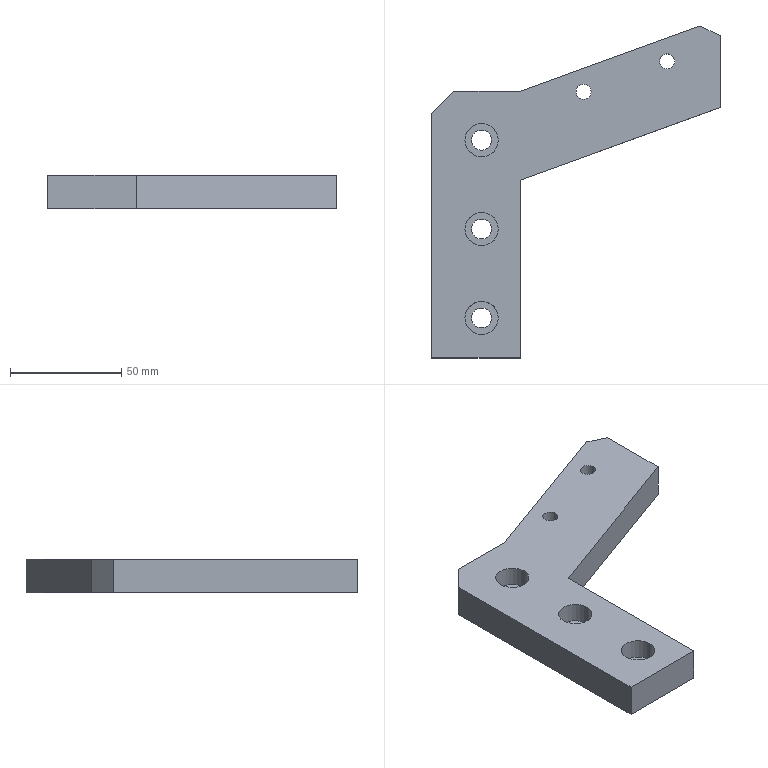Part | SolidWorks | features BaseBody 1 | 1 solid | 30 faces | box 130 x 149.337 x 15 mm | volume 117694 mm3 | cylinder 16 | plane 14 | commonest cylinder face diameters 9 x6 15 x6 6.8 x4
STEP:
#1=CARTESIAN_POINT('',(109.4,133.38,15.));
#2=VERTEX_POINT('',#1);
#3=CARTESIAN_POINT('',(102.6,133.38,15.));
#4=VERTEX_POINT('',#3);
#5=CARTESIAN_POINT('',(106.,133.38,15.));
#6=DIRECTION('',(0.,0.,-1.));
#7=DIRECTION('',(-1.,0.,0.));
#8=AXIS2_PLACEMENT_3D('',#5,#6,#7);
#9=CIRCLE('',#8,3.4);
#10=EDGE_CURVE('',#2,#4,#9,.T.);
#11=ORIENTED_EDGE('',*,*,#10,.F.);
#12=CARTESIAN_POINT('',(109.4,133.38,0.));
#13=VERTEX_POINT('',#12);
#14=CARTESIAN_POINT('',(109.4,133.38,0.));
#15=DIRECTION('',(0.,0.,-1.));
#16=VECTOR('',#15,1000.);
#17=LINE('',#14,#16);
#18=EDGE_CURVE('',#2,#13,#17,.T.);
#19=ORIENTED_EDGE('',*,*,#18,.T.);
#20=CARTESIAN_POINT('',(102.6,133.38,0.));
#21=VERTEX_POINT('',#20);
#22=CARTESIAN_POINT('',(106.,133.38,0.));
#23=DIRECTION('',(0.,0.,-1.));
#24=DIRECTION('',(-1.,0.,0.));
#25=AXIS2_PLACEMENT_3D('',#22,#23,#24);
#26=CIRCLE('',#25,3.4);
#27=EDGE_CURVE('',#13,#21,#26,.T.);
#28=ORIENTED_EDGE('',*,*,#27,.T.);
#29=CARTESIAN_POINT('',(102.6,133.38,0.));
#30=DIRECTION('',(0.,0.,-1.));
#31=VECTOR('',#30,1000.);
#32=LINE('',#29,#31);
#33=EDGE_CURVE('',#4,#21,#32,.T.);
#34=ORIENTED_EDGE('',*,*,#33,.F.);
#35=EDGE_LOOP('',(#11,#19,#28,#34));
#36=FACE_OUTER_BOUND('',#35,.T.);
#37=CARTESIAN_POINT('',(106.,133.38,0.));
#38=DIRECTION('',(0.,0.,-1.));
#39=DIRECTION('',(-1.,0.,0.));
#40=AXIS2_PLACEMENT_3D('',#37,#38,#39);
#41=CYLINDRICAL_SURFACE('',#40,3.4);
#42=ADVANCED_FACE('',(#36),#41,.F.);
#43=CARTESIAN_POINT('',(71.812,119.699,15.));
#44=VERTEX_POINT('',#43);
#45=CARTESIAN_POINT('',(65.012,119.699,15.));
#46=VERTEX_POINT('',#45);
#47=CARTESIAN_POINT('',(68.412,119.699,15.));
#48=DIRECTION('',(0.,0.,-1.));
#49=DIRECTION('',(-1.,0.,0.));
#50=AXIS2_PLACEMENT_3D('',#47,#48,#49);
#51=CIRCLE('',#50,3.4);
#52=EDGE_CURVE('',#44,#46,#51,.T.);
#53=ORIENTED_EDGE('',*,*,#52,.F.);
#54=CARTESIAN_POINT('',(71.812,119.699,0.));
#55=VERTEX_POINT('',#54);
#56=CARTESIAN_POINT('',(71.812,119.699,0.));
#57=DIRECTION('',(0.,0.,-1.));
#58=VECTOR('',#57,1000.);
#59=LINE('',#56,#58);
#60=EDGE_CURVE('',#44,#55,#59,.T.);
#61=ORIENTED_EDGE('',*,*,#60,.T.);
#62=CARTESIAN_POINT('',(65.012,119.699,0.));
#63=VERTEX_POINT('',#62);
#64=CARTESIAN_POINT('',(68.412,119.699,0.));
#65=DIRECTION('',(0.,0.,-1.));
#66=DIRECTION('',(-1.,0.,0.));
#67=AXIS2_PLACEMENT_3D('',#64,#65,#66);
#68=CIRCLE('',#67,3.4);
#69=EDGE_CURVE('',#55,#63,#68,.T.);
#70=ORIENTED_EDGE('',*,*,#69,.T.);
#71=CARTESIAN_POINT('',(65.012,119.699,0.));
#72=DIRECTION('',(0.,0.,-1.));
#73=VECTOR('',#72,1000.);
#74=LINE('',#71,#73);
#75=EDGE_CURVE('',#46,#63,#74,.T.);
#76=ORIENTED_EDGE('',*,*,#75,.F.);
#77=EDGE_LOOP('',(#53,#61,#70,#76));
#78=FACE_OUTER_BOUND('',#77,.T.);
#79=CARTESIAN_POINT('',(68.412,119.699,0.));
#80=DIRECTION('',(0.,0.,-1.));
#81=DIRECTION('',(-1.,0.,0.));
#82=AXIS2_PLACEMENT_3D('',#79,#80,#81);
#83=CYLINDRICAL_SURFACE('',#82,3.4);
#84=ADVANCED_FACE('',(#78),#83,.F.);
#85=CARTESIAN_POINT('',(15.,98.,6.));
#86=VERTEX_POINT('',#85);
#87=CARTESIAN_POINT('',(30.,98.,6.));
#88=VERTEX_POINT('',#87);
#89=CARTESIAN_POINT('',(22.5,98.,6.));
#90=DIRECTION('',(0.,0.,1.));
#91=DIRECTION('',(1.,0.,0.));
#92=AXIS2_PLACEMENT_3D('',#89,#90,#91);
#93=CIRCLE('',#92,7.5);
#94=EDGE_CURVE('',#86,#88,#93,.T.);
#95=ORIENTED_EDGE('',*,*,#94,.F.);
#96=CARTESIAN_POINT('',(15.,98.,15.));
#97=VERTEX_POINT('',#96);
#98=CARTESIAN_POINT('',(15.,98.,15.));
#99=DIRECTION('',(0.,0.,1.));
#100=VECTOR('',#99,1000.);
#101=LINE('',#98,#100);
#102=EDGE_CURVE('',#86,#97,#101,.T.);
#103=ORIENTED_EDGE('',*,*,#102,.T.);
#104=CARTESIAN_POINT('',(30.,98.,15.));
#105=VERTEX_POINT('',#104);
#106=CARTESIAN_POINT('',(22.5,98.,15.));
#107=DIRECTION('',(0.,0.,1.));
#108=DIRECTION('',(1.,0.,0.));
#109=AXIS2_PLACEMENT_3D('',#106,#107,#108);
#110=CIRCLE('',#109,7.5);
#111=EDGE_CURVE('',#97,#105,#110,.T.);
#112=ORIENTED_EDGE('',*,*,#111,.T.);
#113=CARTESIAN_POINT('',(30.,98.,15.));
#114=DIRECTION('',(0.,0.,1.));
#115=VECTOR('',#114,1000.);
#116=LINE('',#113,#115);
#117=EDGE_CURVE('',#88,#105,#116,.T.);
#118=ORIENTED_EDGE('',*,*,#117,.F.);
#119=EDGE_LOOP('',(#95,#103,#112,#118));
#120=FACE_OUTER_BOUND('',#119,.T.);
#121=CARTESIAN_POINT('',(22.5,98.,15.));
#122=DIRECTION('',(0.,0.,1.));
#123=DIRECTION('',(1.,0.,0.));
#124=AXIS2_PLACEMENT_3D('',#121,#122,#123);
#125=CYLINDRICAL_SURFACE('',#124,7.5);
#126=ADVANCED_FACE('',(#120),#125,.F.);
#127=CARTESIAN_POINT('',(18.,98.,0.));
#128=VERTEX_POINT('',#127);
#129=CARTESIAN_POINT('',(27.,98.,0.));
#130=VERTEX_POINT('',#129);
#131=CARTESIAN_POINT('',(22.5,98.,0.));
#132=DIRECTION('',(0.,0.,1.));
#133=DIRECTION('',(1.,0.,0.));
#134=AXIS2_PLACEMENT_3D('',#131,#132,#133);
#135=CIRCLE('',#134,4.5);
#136=EDGE_CURVE('',#128,#130,#135,.T.);
#137=ORIENTED_EDGE('',*,*,#136,.F.);
#138=CARTESIAN_POINT('',(18.,98.,6.));
#139=VERTEX_POINT('',#138);
#140=CARTESIAN_POINT('',(18.,98.,15.));
#141=DIRECTION('',(0.,0.,1.));
#142=VECTOR('',#141,1000.);
#143=LINE('',#140,#142);
#144=EDGE_CURVE('',#128,#139,#143,.T.);
#145=ORIENTED_EDGE('',*,*,#144,.T.);
#146=CARTESIAN_POINT('',(27.,98.,6.));
#147=VERTEX_POINT('',#146);
#148=CARTESIAN_POINT('',(22.5,98.,6.));
#149=DIRECTION('',(0.,0.,1.));
#150=DIRECTION('',(1.,0.,0.));
#151=AXIS2_PLACEMENT_3D('',#148,#149,#150);
#152=CIRCLE('',#151,4.5);
#153=EDGE_CURVE('',#139,#147,#152,.T.);
#154=ORIENTED_EDGE('',*,*,#153,.T.);
#155=CARTESIAN_POINT('',(27.,98.,15.));
#156=DIRECTION('',(0.,0.,1.));
#157=VECTOR('',#156,1000.);
#158=LINE('',#155,#157);
#159=EDGE_CURVE('',#130,#147,#158,.T.);
#160=ORIENTED_EDGE('',*,*,#159,.F.);
#161=EDGE_LOOP('',(#137,#145,#154,#160));
#162=FACE_OUTER_BOUND('',#161,.T.);
#163=CARTESIAN_POINT('',(22.5,98.,15.));
#164=DIRECTION('',(0.,0.,1.));
#165=DIRECTION('',(1.,0.,0.));
#166=AXIS2_PLACEMENT_3D('',#163,#164,#165);
#167=CYLINDRICAL_SURFACE('',#166,4.5);
#168=ADVANCED_FACE('',(#162),#167,.F.);
#169=CARTESIAN_POINT('',(15.,58.,6.));
#170=VERTEX_POINT('',#169);
#171=CARTESIAN_POINT('',(30.,58.,6.));
#172=VERTEX_POINT('',#171);
#173=CARTESIAN_POINT('',(22.5,58.,6.));
#174=DIRECTION('',(0.,0.,1.));
#175=DIRECTION('',(1.,0.,0.));
#176=AXIS2_PLACEMENT_3D('',#173,#174,#175);
#177=CIRCLE('',#176,7.5);
#178=EDGE_CURVE('',#170,#172,#177,.T.);
#179=ORIENTED_EDGE('',*,*,#178,.F.);
#180=CARTESIAN_POINT('',(15.,58.,15.));
#181=VERTEX_POINT('',#180);
#182=CARTESIAN_POINT('',(15.,58.,15.));
#183=DIRECTION('',(0.,0.,1.));
#184=VECTOR('',#183,1000.);
#185=LINE('',#182,#184);
#186=EDGE_CURVE('',#170,#181,#185,.T.);
#187=ORIENTED_EDGE('',*,*,#186,.T.);
#188=CARTESIAN_POINT('',(30.,58.,15.));
#189=VERTEX_POINT('',#188);
#190=CARTESIAN_POINT('',(22.5,58.,15.));
#191=DIRECTION('',(0.,0.,1.));
#192=DIRECTION('',(1.,0.,0.));
#193=AXIS2_PLACEMENT_3D('',#190,#191,#192);
#194=CIRCLE('',#193,7.5);
#195=EDGE_CURVE('',#181,#189,#194,.T.);
#196=ORIENTED_EDGE('',*,*,#195,.T.);
#197=CARTESIAN_POINT('',(30.,58.,15.));
#198=DIRECTION('',(0.,0.,1.));
#199=VECTOR('',#198,1000.);
#200=LINE('',#197,#199);
#201=EDGE_CURVE('',#172,#189,#200,.T.);
#202=ORIENTED_EDGE('',*,*,#201,.F.);
#203=EDGE_LOOP('',(#179,#187,#196,#202));
#204=FACE_OUTER_BOUND('',#203,.T.);
#205=CARTESIAN_POINT('',(22.5,58.,15.));
#206=DIRECTION('',(0.,0.,1.));
#207=DIRECTION('',(1.,0.,0.));
#208=AXIS2_PLACEMENT_3D('',#205,#206,#207);
#209=CYLINDRICAL_SURFACE('',#208,7.5);
#210=ADVANCED_FACE('',(#204),#209,.F.);
#211=CARTESIAN_POINT('',(18.,58.,0.));
#212=VERTEX_POINT('',#211);
#213=CARTESIAN_POINT('',(27.,58.,0.));
#214=VERTEX_POINT('',#213);
#215=CARTESIAN_POINT('',(22.5,58.,0.));
#216=DIRECTION('',(0.,0.,1.));
#217=DIRECTION('',(1.,0.,0.));
#218=AXIS2_PLACEMENT_3D('',#215,#216,#217);
#219=CIRCLE('',#218,4.5);
#220=EDGE_CURVE('',#212,#214,#219,.T.);
#221=ORIENTED_EDGE('',*,*,#220,.F.);
#222=CARTESIAN_POINT('',(18.,58.,6.));
#223=VERTEX_POINT('',#222);
#224=CARTESIAN_POINT('',(18.,58.,15.));
#225=DIRECTION('',(0.,0.,1.));
#226=VECTOR('',#225,1000.);
#227=LINE('',#224,#226);
#228=EDGE_CURVE('',#212,#223,#227,.T.);
#229=ORIENTED_EDGE('',*,*,#228,.T.);
#230=CARTESIAN_POINT('',(27.,58.,6.));
#231=VERTEX_POINT('',#230);
#232=CARTESIAN_POINT('',(22.5,58.,6.));
#233=DIRECTION('',(0.,0.,1.));
#234=DIRECTION('',(1.,0.,0.));
#235=AXIS2_PLACEMENT_3D('',#232,#233,#234);
#236=CIRCLE('',#235,4.5);
#237=EDGE_CURVE('',#223,#231,#236,.T.);
#238=ORIENTED_EDGE('',*,*,#237,.T.);
#239=CARTESIAN_POINT('',(27.,58.,15.));
#240=DIRECTION('',(0.,0.,1.));
#241=VECTOR('',#240,1000.);
#242=LINE('',#239,#241);
#243=EDGE_CURVE('',#214,#231,#242,.T.);
#244=ORIENTED_EDGE('',*,*,#243,.F.);
#245=EDGE_LOOP('',(#221,#229,#238,#244));
#246=FACE_OUTER_BOUND('',#245,.T.);
#247=CARTESIAN_POINT('',(22.5,58.,15.));
#248=DIRECTION('',(0.,0.,1.));
#249=DIRECTION('',(1.,0.,0.));
#250=AXIS2_PLACEMENT_3D('',#247,#248,#249);
#251=CYLINDRICAL_SURFACE('',#250,4.5);
#252=ADVANCED_FACE('',(#246),#251,.F.);
#253=CARTESIAN_POINT('',(15.,18.,6.));
#254=VERTEX_POINT('',#253);
#255=CARTESIAN_POINT('',(30.,18.,6.));
#256=VERTEX_POINT('',#255);
#257=CARTESIAN_POINT('',(22.5,18.,6.));
#258=DIRECTION('',(0.,0.,1.));
#259=DIRECTION('',(1.,0.,0.));
#260=AXIS2_PLACEMENT_3D('',#257,#258,#259);
#261=CIRCLE('',#260,7.5);
#262=EDGE_CURVE('',#254,#256,#261,.T.);
#263=ORIENTED_EDGE('',*,*,#262,.F.);
#264=CARTESIAN_POINT('',(15.,18.,15.));
#265=VERTEX_POINT('',#264);
#266=CARTESIAN_POINT('',(15.,18.,15.));
#267=DIRECTION('',(0.,0.,1.));
#268=VECTOR('',#267,1000.);
#269=LINE('',#266,#268);
#270=EDGE_CURVE('',#254,#265,#269,.T.);
#271=ORIENTED_EDGE('',*,*,#270,.T.);
#272=CARTESIAN_POINT('',(30.,18.,15.));
#273=VERTEX_POINT('',#272);
#274=CARTESIAN_POINT('',(22.5,18.,15.));
#275=DIRECTION('',(0.,0.,1.));
#276=DIRECTION('',(1.,0.,0.));
#277=AXIS2_PLACEMENT_3D('',#274,#275,#276);
#278=CIRCLE('',#277,7.5);
#279=EDGE_CURVE('',#265,#273,#278,.T.);
#280=ORIENTED_EDGE('',*,*,#279,.T.);
#281=CARTESIAN_POINT('',(30.,18.,15.));
#282=DIRECTION('',(0.,0.,1.));
#283=VECTOR('',#282,1000.);
#284=LINE('',#281,#283);
#285=EDGE_CURVE('',#256,#273,#284,.T.);
#286=ORIENTED_EDGE('',*,*,#285,.F.);
#287=EDGE_LOOP('',(#263,#271,#280,#286));
#288=FACE_OUTER_BOUND('',#287,.T.);
#289=CARTESIAN_POINT('',(22.5,18.,15.));
#290=DIRECTION('',(0.,0.,1.));
#291=DIRECTION('',(1.,0.,0.));
#292=AXIS2_PLACEMENT_3D('',#289,#290,#291);
#293=CYLINDRICAL_SURFACE('',#292,7.5);
#294=ADVANCED_FACE('',(#288),#293,.F.);
#295=CARTESIAN_POINT('',(18.,18.,0.));
#296=VERTEX_POINT('',#295);
#297=CARTESIAN_POINT('',(27.,18.,0.));
#298=VERTEX_POINT('',#297);
#299=CARTESIAN_POINT('',(22.5,18.,0.));
#300=DIRECTION('',(0.,0.,1.));
#301=DIRECTION('',(1.,0.,0.));
#302=AXIS2_PLACEMENT_3D('',#299,#300,#301);
#303=CIRCLE('',#302,4.5);
#304=EDGE_CURVE('',#296,#298,#303,.T.);
#305=ORIENTED_EDGE('',*,*,#304,.F.);
#306=CARTESIAN_POINT('',(18.,18.,6.));
#307=VERTEX_POINT('',#306);
#308=CARTESIAN_POINT('',(18.,18.,15.));
#309=DIRECTION('',(0.,0.,1.));
#310=VECTOR('',#309,1000.);
#311=LINE('',#308,#310);
#312=EDGE_CURVE('',#296,#307,#311,.T.);
#313=ORIENTED_EDGE('',*,*,#312,.T.);
#314=CARTESIAN_POINT('',(27.,18.,6.));
#315=VERTEX_POINT('',#314);
#316=CARTESIAN_POINT('',(22.5,18.,6.));
#317=DIRECTION('',(0.,0.,1.));
#318=DIRECTION('',(1.,0.,0.));
#319=AXIS2_PLACEMENT_3D('',#316,#317,#318);
#320=CIRCLE('',#319,4.5);
#321=EDGE_CURVE('',#307,#315,#320,.T.);
#322=ORIENTED_EDGE('',*,*,#321,.T.);
#323=CARTESIAN_POINT('',(27.,18.,15.));
#324=DIRECTION('',(0.,0.,1.));
#325=VECTOR('',#324,1000.);
#326=LINE('',#323,#325);
#327=EDGE_CURVE('',#298,#315,#326,.T.);
#328=ORIENTED_EDGE('',*,*,#327,.F.);
#329=EDGE_LOOP('',(#305,#313,#322,#328));
#330=FACE_OUTER_BOUND('',#329,.T.);
#331=CARTESIAN_POINT('',(22.5,18.,15.));
#332=DIRECTION('',(0.,0.,1.));
#333=DIRECTION('',(1.,0.,0.));
#334=AXIS2_PLACEMENT_3D('',#331,#332,#333);
#335=CYLINDRICAL_SURFACE('',#334,4.5);
#336=ADVANCED_FACE('',(#330),#335,.F.);
#337=CARTESIAN_POINT('',(0.,110.,0.));
#338=VERTEX_POINT('',#337);
#339=CARTESIAN_POINT('',(10.,120.,0.));
#340=VERTEX_POINT('',#339);
#341=CARTESIAN_POINT('',(-55.,55.,0.));
#342=DIRECTION('',(0.7071,0.7071,0.));
#343=VECTOR('',#342,1000.);
#344=LINE('',#341,#343);
#345=EDGE_CURVE('',#338,#340,#344,.T.);
#346=ORIENTED_EDGE('',*,*,#345,.F.);
#347=CARTESIAN_POINT('',(0.,110.,15.));
#348=VERTEX_POINT('',#347);
#349=CARTESIAN_POINT('',(0.,110.,15.));
#350=DIRECTION('',(0.,0.,-1.));
#351=VECTOR('',#350,1000.);
#352=LINE('',#349,#351);
#353=EDGE_CURVE('',#348,#338,#352,.T.);
#354=ORIENTED_EDGE('',*,*,#353,.F.);
#355=CARTESIAN_POINT('',(10.,120.,15.));
#356=VERTEX_POINT('',#355);
#357=CARTESIAN_POINT('',(10.,120.,15.));
#358=DIRECTION('',(-0.7071,-0.7071,0.));
#359=VECTOR('',#358,1000.);
#360=LINE('',#357,#359);
#361=EDGE_CURVE('',#356,#348,#360,.T.);
#362=ORIENTED_EDGE('',*,*,#361,.F.);
#363=CARTESIAN_POINT('',(10.,120.,0.));
#364=DIRECTION('',(0.,0.,1.));
#365=VECTOR('',#364,1000.);
#366=LINE('',#363,#365);
#367=EDGE_CURVE('',#340,#356,#366,.T.);
#368=ORIENTED_EDGE('',*,*,#367,.F.);
#369=EDGE_LOOP('',(#346,#354,#362,#368));
#370=FACE_OUTER_BOUND('',#369,.T.);
#371=CARTESIAN_POINT('',(10.,120.,0.));
#372=DIRECTION('',(0.7071,-0.7071,0.));
#373=DIRECTION('',(0.,0.,-1.));
#374=AXIS2_PLACEMENT_3D('',#371,#372,#373);
#375=PLANE('',#374);
#376=ADVANCED_FACE('',(#370),#375,.F.);
#377=CARTESIAN_POINT('',(120.603,149.337,0.));
#378=VERTEX_POINT('',#377);
#379=CARTESIAN_POINT('',(130.,144.955,0.));
#380=VERTEX_POINT('',#379);
#381=CARTESIAN_POINT('',(78.74,168.858,0.));
#382=DIRECTION('',(0.9063,-0.4226,0.));
#383=VECTOR('',#382,1000.);
#384=LINE('',#381,#383);
#385=EDGE_CURVE('',#378,#380,#384,.T.);
#386=ORIENTED_EDGE('',*,*,#385,.F.);
#387=CARTESIAN_POINT('',(120.603,149.337,15.));
#388=VERTEX_POINT('',#387);
#389=CARTESIAN_POINT('',(120.603,149.337,0.));
#390=DIRECTION('',(0.,0.,-1.));
#391=VECTOR('',#390,1000.);
#392=LINE('',#389,#391);
#393=EDGE_CURVE('',#388,#378,#392,.T.);
#394=ORIENTED_EDGE('',*,*,#393,.F.);
#395=CARTESIAN_POINT('',(130.,144.955,15.));
#396=VERTEX_POINT('',#395);
#397=CARTESIAN_POINT('',(130.,144.955,15.));
#398=DIRECTION('',(-0.9063,0.4226,0.));
#399=VECTOR('',#398,1000.);
#400=LINE('',#397,#399);
#401=EDGE_CURVE('',#396,#388,#400,.T.);
#402=ORIENTED_EDGE('',*,*,#401,.F.);
#403=CARTESIAN_POINT('',(130.,144.955,15.));
#404=DIRECTION('',(0.,0.,1.));
#405=VECTOR('',#404,1000.);
#406=LINE('',#403,#405);
#407=EDGE_CURVE('',#380,#396,#406,.T.);
#408=ORIENTED_EDGE('',*,*,#407,.F.);
#409=EDGE_LOOP('',(#386,#394,#402,#408));
#410=FACE_OUTER_BOUND('',#409,.T.);
#411=CARTESIAN_POINT('',(130.,144.955,15.));
#412=DIRECTION('',(-0.4226,-0.9063,0.));
#413=DIRECTION('',(-0.9063,0.4226,0.));
#414=AXIS2_PLACEMENT_3D('',#411,#412,#413);
#415=PLANE('',#414);
#416=ADVANCED_FACE('',(#410),#415,.F.);
#417=CARTESIAN_POINT('',(22.5,98.,6.));
#418=DIRECTION('',(0.,0.,1.));
#419=DIRECTION('',(1.,0.,0.));
#420=AXIS2_PLACEMENT_3D('',#417,#418,#419);
#421=CIRCLE('',#420,4.5);
#422=EDGE_CURVE('',#147,#139,#421,.T.);
#423=ORIENTED_EDGE('',*,*,#422,.F.);
#424=ORIENTED_EDGE('',*,*,#153,.F.);
#425=EDGE_LOOP('',(#423,#424));
#426=FACE_BOUND('',#425,.T.);
#427=CARTESIAN_POINT('',(22.5,98.,6.));
#428=DIRECTION('',(0.,0.,1.));
#429=DIRECTION('',(1.,0.,0.));
#430=AXIS2_PLACEMENT_3D('',#427,#428,#429);
#431=CIRCLE('',#430,7.5);
#432=EDGE_CURVE('',#88,#86,#431,.T.);
#433=ORIENTED_EDGE('',*,*,#432,.T.);
#434=ORIENTED_EDGE('',*,*,#94,.T.);
#435=EDGE_LOOP('',(#433,#434));
#436=FACE_OUTER_BOUND('',#435,.T.);
#437=CARTESIAN_POINT('',(27.,98.,6.));
#438=DIRECTION('',(0.,0.,-1.));
#439=DIRECTION('',(0.,-1.,0.));
#440=AXIS2_PLACEMENT_3D('',#437,#438,#439);
#441=PLANE('',#440);
#442=ADVANCED_FACE('',(#426,#436),#441,.F.);
#443=CARTESIAN_POINT('',(22.5,58.,6.));
#444=DIRECTION('',(0.,0.,1.));
#445=DIRECTION('',(1.,0.,0.));
#446=AXIS2_PLACEMENT_3D('',#443,#444,#445);
#447=CIRCLE('',#446,4.5);
#448=EDGE_CURVE('',#231,#223,#447,.T.);
#449=ORIENTED_EDGE('',*,*,#448,.F.);
#450=ORIENTED_EDGE('',*,*,#237,.F.);
#451=EDGE_LOOP('',(#449,#450));
#452=FACE_BOUND('',#451,.T.);
#453=CARTESIAN_POINT('',(22.5,58.,6.));
#454=DIRECTION('',(0.,0.,1.));
#455=DIRECTION('',(1.,0.,0.));
#456=AXIS2_PLACEMENT_3D('',#453,#454,#455);
#457=CIRCLE('',#456,7.5);
#458=EDGE_CURVE('',#172,#170,#457,.T.);
#459=ORIENTED_EDGE('',*,*,#458,.T.);
#460=ORIENTED_EDGE('',*,*,#178,.T.);
#461=EDGE_LOOP('',(#459,#460));
#462=FACE_OUTER_BOUND('',#461,.T.);
#463=CARTESIAN_POINT('',(27.,58.,6.));
#464=DIRECTION('',(0.,0.,-1.));
#465=DIRECTION('',(0.,-1.,0.));
#466=AXIS2_PLACEMENT_3D('',#463,#464,#465);
#467=PLANE('',#466);
#468=ADVANCED_FACE('',(#452,#462),#467,.F.);
#469=CARTESIAN_POINT('',(22.5,18.,6.));
#470=DIRECTION('',(0.,0.,1.));
#471=DIRECTION('',(1.,0.,0.));
#472=AXIS2_PLACEMENT_3D('',#469,#470,#471);
#473=CIRCLE('',#472,4.5);
#474=EDGE_CURVE('',#315,#307,#473,.T.);
#475=ORIENTED_EDGE('',*,*,#474,.F.);
#476=ORIENTED_EDGE('',*,*,#321,.F.);
#477=EDGE_LOOP('',(#475,#476));
#478=FACE_BOUND('',#477,.T.);
#479=CARTESIAN_POINT('',(22.5,18.,6.));
#480=DIRECTION('',(0.,0.,1.));
#481=DIRECTION('',(1.,0.,0.));
#482=AXIS2_PLACEMENT_3D('',#479,#480,#481);
#483=CIRCLE('',#482,7.5);
#484=EDGE_CURVE('',#256,#254,#483,.T.);
#485=ORIENTED_EDGE('',*,*,#484,.T.);
#486=ORIENTED_EDGE('',*,*,#262,.T.);
#487=EDGE_LOOP('',(#485,#486));
#488=FACE_OUTER_BOUND('',#487,.T.);
#489=CARTESIAN_POINT('',(27.,18.,6.));
#490=DIRECTION('',(0.,0.,-1.));
#491=DIRECTION('',(0.,-1.,0.));
#492=AXIS2_PLACEMENT_3D('',#489,#490,#491);
#493=PLANE('',#492);
#494=ADVANCED_FACE('',(#478,#488),#493,.F.);
#495=CARTESIAN_POINT('',(130.,112.757,15.));
#496=VERTEX_POINT('',#495);
#497=CARTESIAN_POINT('',(40.,80.,15.));
#498=VERTEX_POINT('',#497);
#499=CARTESIAN_POINT('',(130.,112.757,15.));
#500=DIRECTION('',(-0.9397,-0.342,0.));
#501=VECTOR('',#500,1000.);
#502=LINE('',#499,#501);
#503=EDGE_CURVE('',#496,#498,#502,.T.);
#504=ORIENTED_EDGE('',*,*,#503,.T.);
#505=CARTESIAN_POINT('',(40.,80.,0.));
#506=VERTEX_POINT('',#505);
#507=CARTESIAN_POINT('',(40.,80.,0.));
#508=DIRECTION('',(0.,0.,1.));
#509=VECTOR('',#508,1000.);
#510=LINE('',#507,#509);
#511=EDGE_CURVE('',#506,#498,#510,.T.);
#512=ORIENTED_EDGE('',*,*,#511,.F.);
#513=CARTESIAN_POINT('',(130.,112.757,0.));
#514=VERTEX_POINT('',#513);
#515=CARTESIAN_POINT('',(130.,112.757,0.));
#516=DIRECTION('',(-0.9397,-0.342,0.));
#517=VECTOR('',#516,1000.);
#518=LINE('',#515,#517);
#519=EDGE_CURVE('',#514,#506,#518,.T.);
#520=ORIENTED_EDGE('',*,*,#519,.F.);
#521=CARTESIAN_POINT('',(130.,112.757,0.));
#522=DIRECTION('',(0.,0.,1.));
#523=VECTOR('',#522,1000.);
#524=LINE('',#521,#523);
#525=EDGE_CURVE('',#514,#496,#524,.T.);
#526=ORIENTED_EDGE('',*,*,#525,.T.);
#527=EDGE_LOOP('',(#504,#512,#520,#526));
#528=FACE_OUTER_BOUND('',#527,.T.);
#529=CARTESIAN_POINT('',(130.,112.757,0.));
#530=DIRECTION('',(-0.342,0.9397,0.));
#531=DIRECTION('',(0.,0.,1.));
#532=AXIS2_PLACEMENT_3D('',#529,#530,#531);
#533=PLANE('',#532);
#534=ADVANCED_FACE('',(#528),#533,.F.);
#535=CARTESIAN_POINT('',(40.,0.,15.));
#536=VERTEX_POINT('',#535);
#537=CARTESIAN_POINT('',(40.,80.,15.));
#538=DIRECTION('',(0.,-1.,0.));
#539=VECTOR('',#538,1000.);
#540=LINE('',#537,#539);
#541=EDGE_CURVE('',#498,#536,#540,.T.);
#542=ORIENTED_EDGE('',*,*,#541,.T.);
#543=CARTESIAN_POINT('',(40.,0.,0.));
#544=VERTEX_POINT('',#543);
#545=CARTESIAN_POINT('',(40.,0.,0.));
#546=DIRECTION('',(0.,0.,1.));
#547=VECTOR('',#546,1000.);
#548=LINE('',#545,#547);
#549=EDGE_CURVE('',#544,#536,#548,.T.);
#550=ORIENTED_EDGE('',*,*,#549,.F.);
#551=CARTESIAN_POINT('',(40.,80.,0.));
#552=DIRECTION('',(0.,-1.,0.));
#553=VECTOR('',#552,1000.);
#554=LINE('',#551,#553);
#555=EDGE_CURVE('',#506,#544,#554,.T.);
#556=ORIENTED_EDGE('',*,*,#555,.F.);
#557=ORIENTED_EDGE('',*,*,#511,.T.);
#558=EDGE_LOOP('',(#542,#550,#556,#557));
#559=FACE_OUTER_BOUND('',#558,.T.);
#560=CARTESIAN_POINT('',(40.,80.,0.));
#561=DIRECTION('',(-1.,0.,0.));
#562=DIRECTION('',(0.,1.,0.));
#563=AXIS2_PLACEMENT_3D('',#560,#561,#562);
#564=PLANE('',#563);
#565=ADVANCED_FACE('',(#559),#564,.F.);
#566=CARTESIAN_POINT('',(40.,120.,0.));
#567=VERTEX_POINT('',#566);
#568=CARTESIAN_POINT('',(0.,120.,0.));
#569=DIRECTION('',(1.,0.,0.));
#570=VECTOR('',#569,1000.);
#571=LINE('',#568,#570);
#572=EDGE_CURVE('',#340,#567,#571,.T.);
#573=ORIENTED_EDGE('',*,*,#572,.F.);
#574=ORIENTED_EDGE('',*,*,#367,.T.);
#575=CARTESIAN_POINT('',(40.,120.,15.));
#576=VERTEX_POINT('',#575);
#577=CARTESIAN_POINT('',(0.,120.,15.));
#578=DIRECTION('',(1.,0.,0.));
#579=VECTOR('',#578,1000.);
#580=LINE('',#577,#579);
#581=EDGE_CURVE('',#356,#576,#580,.T.);
#582=ORIENTED_EDGE('',*,*,#581,.T.);
#583=CARTESIAN_POINT('',(40.,120.,0.));
#584=DIRECTION('',(0.,0.,1.));
#585=VECTOR('',#584,1000.);
#586=LINE('',#583,#585);
#587=EDGE_CURVE('',#567,#576,#586,.T.);
#588=ORIENTED_EDGE('',*,*,#587,.F.);
#589=EDGE_LOOP('',(#573,#574,#582,#588));
#590=FACE_OUTER_BOUND('',#589,.T.);
#591=CARTESIAN_POINT('',(0.,120.,0.));
#592=DIRECTION('',(0.,-1.,0.));
#593=DIRECTION('',(0.,0.,-1.));
#594=AXIS2_PLACEMENT_3D('',#591,#592,#593);
#595=PLANE('',#594);
#596=ADVANCED_FACE('',(#590),#595,.F.);
#597=CARTESIAN_POINT('',(40.,120.,15.));
#598=DIRECTION('',(0.9397,0.342,0.));
#599=VECTOR('',#598,1000.);
#600=LINE('',#597,#599);
#601=EDGE_CURVE('',#576,#388,#600,.T.);
#602=ORIENTED_EDGE('',*,*,#601,.T.);
#603=ORIENTED_EDGE('',*,*,#393,.T.);
#604=CARTESIAN_POINT('',(40.,120.,0.));
#605=DIRECTION('',(0.9397,0.342,0.));
#606=VECTOR('',#605,1000.);
#607=LINE('',#604,#606);
#608=EDGE_CURVE('',#567,#378,#607,.T.);
#609=ORIENTED_EDGE('',*,*,#608,.F.);
#610=ORIENTED_EDGE('',*,*,#587,.T.);
#611=EDGE_LOOP('',(#602,#603,#609,#610));
#612=FACE_OUTER_BOUND('',#611,.T.);
#613=CARTESIAN_POINT('',(40.,120.,0.));
#614=DIRECTION('',(0.342,-0.9397,0.));
#615=DIRECTION('',(0.,0.,-1.));
#616=AXIS2_PLACEMENT_3D('',#613,#614,#615);
#617=PLANE('',#616);
#618=ADVANCED_FACE('',(#612),#617,.F.);
#619=CARTESIAN_POINT('',(22.5,18.,0.));
#620=DIRECTION('',(0.,0.,1.));
#621=DIRECTION('',(1.,0.,0.));
#622=AXIS2_PLACEMENT_3D('',#619,#620,#621);
#623=CIRCLE('',#622,4.5);
#624=EDGE_CURVE('',#298,#296,#623,.T.);
#625=ORIENTED_EDGE('',*,*,#624,.T.);
#626=ORIENTED_EDGE('',*,*,#304,.T.);
#627=EDGE_LOOP('',(#625,#626));
#628=FACE_BOUND('',#627,.T.);
#629=CARTESIAN_POINT('',(22.5,58.,0.));
#630=DIRECTION('',(0.,0.,1.));
#631=DIRECTION('',(1.,0.,0.));
#632=AXIS2_PLACEMENT_3D('',#629,#630,#631);
#633=CIRCLE('',#632,4.5);
#634=EDGE_CURVE('',#214,#212,#633,.T.);
#635=ORIENTED_EDGE('',*,*,#634,.T.);
#636=ORIENTED_EDGE('',*,*,#220,.T.);
#637=EDGE_LOOP('',(#635,#636));
#638=FACE_BOUND('',#637,.T.);
#639=CARTESIAN_POINT('',(22.5,98.,0.));
#640=DIRECTION('',(0.,0.,1.));
#641=DIRECTION('',(1.,0.,0.));
#642=AXIS2_PLACEMENT_3D('',#639,#640,#641);
#643=CIRCLE('',#642,4.5);
#644=EDGE_CURVE('',#130,#128,#643,.T.);
#645=ORIENTED_EDGE('',*,*,#644,.T.);
#646=ORIENTED_EDGE('',*,*,#136,.T.);
#647=EDGE_LOOP('',(#645,#646));
#648=FACE_BOUND('',#647,.T.);
#649=CARTESIAN_POINT('',(68.412,119.699,0.));
#650=DIRECTION('',(0.,0.,-1.));
#651=DIRECTION('',(-1.,0.,0.));
#652=AXIS2_PLACEMENT_3D('',#649,#650,#651);
#653=CIRCLE('',#652,3.4);
#654=EDGE_CURVE('',#63,#55,#653,.T.);
#655=ORIENTED_EDGE('',*,*,#654,.F.);
#656=ORIENTED_EDGE('',*,*,#69,.F.);
#657=EDGE_LOOP('',(#655,#656));
#658=FACE_BOUND('',#657,.T.);
#659=CARTESIAN_POINT('',(106.,133.38,0.));
#660=DIRECTION('',(0.,0.,-1.));
#661=DIRECTION('',(-1.,0.,0.));
#662=AXIS2_PLACEMENT_3D('',#659,#660,#661);
#663=CIRCLE('',#662,3.4);
#664=EDGE_CURVE('',#21,#13,#663,.T.);
#665=ORIENTED_EDGE('',*,*,#664,.F.);
#666=ORIENTED_EDGE('',*,*,#27,.F.);
#667=EDGE_LOOP('',(#665,#666));
#668=FACE_BOUND('',#667,.T.);
#669=CARTESIAN_POINT('',(0.,0.,0.));
#670=VERTEX_POINT('',#669);
#671=CARTESIAN_POINT('',(0.,0.,0.));
#672=DIRECTION('',(0.,-1.,0.));
#673=VECTOR('',#672,1000.);
#674=LINE('',#671,#673);
#675=EDGE_CURVE('',#338,#670,#674,.T.);
#676=ORIENTED_EDGE('',*,*,#675,.F.);
#677=ORIENTED_EDGE('',*,*,#345,.T.);
#678=ORIENTED_EDGE('',*,*,#572,.T.);
#679=ORIENTED_EDGE('',*,*,#608,.T.);
#680=ORIENTED_EDGE('',*,*,#385,.T.);
#681=CARTESIAN_POINT('',(130.,0.,0.));
#682=DIRECTION('',(0.,1.,0.));
#683=VECTOR('',#682,1000.);
#684=LINE('',#681,#683);
#685=EDGE_CURVE('',#514,#380,#684,.T.);
#686=ORIENTED_EDGE('',*,*,#685,.F.);
#687=ORIENTED_EDGE('',*,*,#519,.T.);
#688=ORIENTED_EDGE('',*,*,#555,.T.);
#689=CARTESIAN_POINT('',(0.,0.,0.));
#690=DIRECTION('',(1.,0.,0.));
#691=VECTOR('',#690,1000.);
#692=LINE('',#689,#691);
#693=EDGE_CURVE('',#670,#544,#692,.T.);
#694=ORIENTED_EDGE('',*,*,#693,.F.);
#695=EDGE_LOOP('',(#676,#677,#678,#679,#680,#686,#687,#688,#694));
#696=FACE_OUTER_BOUND('',#695,.T.);
#697=CARTESIAN_POINT('',(0.,0.,0.));
#698=DIRECTION('',(0.,0.,-1.));
#699=DIRECTION('',(0.,-1.,0.));
#700=AXIS2_PLACEMENT_3D('',#697,#698,#699);
#701=PLANE('',#700);
#702=ADVANCED_FACE('',(#628,#638,#648,#658,#668,#696),#701,.T.);
#703=CARTESIAN_POINT('',(22.5,18.,15.));
#704=DIRECTION('',(0.,0.,1.));
#705=DIRECTION('',(1.,0.,0.));
#706=AXIS2_PLACEMENT_3D('',#703,#704,#705);
#707=CIRCLE('',#706,7.5);
#708=EDGE_CURVE('',#273,#265,#707,.T.);
#709=ORIENTED_EDGE('',*,*,#708,.F.);
#710=ORIENTED_EDGE('',*,*,#279,.F.);
#711=EDGE_LOOP('',(#709,#710));
#712=FACE_BOUND('',#711,.T.);
#713=CARTESIAN_POINT('',(22.5,58.,15.));
#714=DIRECTION('',(0.,0.,1.));
#715=DIRECTION('',(1.,0.,0.));
#716=AXIS2_PLACEMENT_3D('',#713,#714,#715);
#717=CIRCLE('',#716,7.5);
#718=EDGE_CURVE('',#189,#181,#717,.T.);
#719=ORIENTED_EDGE('',*,*,#718,.F.);
#720=ORIENTED_EDGE('',*,*,#195,.F.);
#721=EDGE_LOOP('',(#719,#720));
#722=FACE_BOUND('',#721,.T.);
#723=CARTESIAN_POINT('',(22.5,98.,15.));
#724=DIRECTION('',(0.,0.,1.));
#725=DIRECTION('',(1.,0.,0.));
#726=AXIS2_PLACEMENT_3D('',#723,#724,#725);
#727=CIRCLE('',#726,7.5);
#728=EDGE_CURVE('',#105,#97,#727,.T.);
#729=ORIENTED_EDGE('',*,*,#728,.F.);
#730=ORIENTED_EDGE('',*,*,#111,.F.);
#731=EDGE_LOOP('',(#729,#730));
#732=FACE_BOUND('',#731,.T.);
#733=CARTESIAN_POINT('',(68.412,119.699,15.));
#734=DIRECTION('',(0.,0.,-1.));
#735=DIRECTION('',(-1.,0.,0.));
#736=AXIS2_PLACEMENT_3D('',#733,#734,#735);
#737=CIRCLE('',#736,3.4);
#738=EDGE_CURVE('',#46,#44,#737,.T.);
#739=ORIENTED_EDGE('',*,*,#738,.T.);
#740=ORIENTED_EDGE('',*,*,#52,.T.);
#741=EDGE_LOOP('',(#739,#740));
#742=FACE_BOUND('',#741,.T.);
#743=CARTESIAN_POINT('',(106.,133.38,15.));
#744=DIRECTION('',(0.,0.,-1.));
#745=DIRECTION('',(-1.,0.,0.));
#746=AXIS2_PLACEMENT_3D('',#743,#744,#745);
#747=CIRCLE('',#746,3.4);
#748=EDGE_CURVE('',#4,#2,#747,.T.);
#749=ORIENTED_EDGE('',*,*,#748,.T.);
#750=ORIENTED_EDGE('',*,*,#10,.T.);
#751=EDGE_LOOP('',(#749,#750));
#752=FACE_BOUND('',#751,.T.);
#753=ORIENTED_EDGE('',*,*,#581,.F.);
#754=ORIENTED_EDGE('',*,*,#361,.T.);
#755=CARTESIAN_POINT('',(0.,0.,15.));
#756=VERTEX_POINT('',#755);
#757=CARTESIAN_POINT('',(0.,0.,15.));
#758=DIRECTION('',(0.,-1.,0.));
#759=VECTOR('',#758,1000.);
#760=LINE('',#757,#759);
#761=EDGE_CURVE('',#348,#756,#760,.T.);
#762=ORIENTED_EDGE('',*,*,#761,.T.);
#763=CARTESIAN_POINT('',(0.,0.,15.));
#764=DIRECTION('',(1.,0.,0.));
#765=VECTOR('',#764,1000.);
#766=LINE('',#763,#765);
#767=EDGE_CURVE('',#756,#536,#766,.T.);
#768=ORIENTED_EDGE('',*,*,#767,.T.);
#769=ORIENTED_EDGE('',*,*,#541,.F.);
#770=ORIENTED_EDGE('',*,*,#503,.F.);
#771=CARTESIAN_POINT('',(130.,0.,15.));
#772=DIRECTION('',(0.,1.,0.));
#773=VECTOR('',#772,1000.);
#774=LINE('',#771,#773);
#775=EDGE_CURVE('',#496,#396,#774,.T.);
#776=ORIENTED_EDGE('',*,*,#775,.T.);
#777=ORIENTED_EDGE('',*,*,#401,.T.);
#778=ORIENTED_EDGE('',*,*,#601,.F.);
#779=EDGE_LOOP('',(#753,#754,#762,#768,#769,#770,#776,#777,#778));
#780=FACE_OUTER_BOUND('',#779,.T.);
#781=CARTESIAN_POINT('',(0.,0.,15.));
#782=DIRECTION('',(0.,0.,-1.));
#783=DIRECTION('',(0.,-1.,0.));
#784=AXIS2_PLACEMENT_3D('',#781,#782,#783);
#785=PLANE('',#784);
#786=ADVANCED_FACE('',(#712,#722,#732,#742,#752,#780),#785,.F.);
#787=ORIENTED_EDGE('',*,*,#685,.T.);
#788=ORIENTED_EDGE('',*,*,#407,.T.);
#789=ORIENTED_EDGE('',*,*,#775,.F.);
#790=ORIENTED_EDGE('',*,*,#525,.F.);
#791=EDGE_LOOP('',(#787,#788,#789,#790));
#792=FACE_OUTER_BOUND('',#791,.T.);
#793=CARTESIAN_POINT('',(130.,0.,15.));
#794=DIRECTION('',(-1.,0.,0.));
#795=DIRECTION('',(0.,0.,1.));
#796=AXIS2_PLACEMENT_3D('',#793,#794,#795);
#797=PLANE('',#796);
#798=ADVANCED_FACE('',(#792),#797,.F.);
#799=ORIENTED_EDGE('',*,*,#693,.T.);
#800=ORIENTED_EDGE('',*,*,#549,.T.);
#801=ORIENTED_EDGE('',*,*,#767,.F.);
#802=CARTESIAN_POINT('',(0.,0.,15.));
#803=DIRECTION('',(0.,0.,-1.));
#804=VECTOR('',#803,1000.);
#805=LINE('',#802,#804);
#806=EDGE_CURVE('',#756,#670,#805,.T.);
#807=ORIENTED_EDGE('',*,*,#806,.T.);
#808=EDGE_LOOP('',(#799,#800,#801,#807));
#809=FACE_OUTER_BOUND('',#808,.T.);
#810=CARTESIAN_POINT('',(0.,0.,15.));
#811=DIRECTION('',(0.,1.,0.));
#812=DIRECTION('',(1.,0.,0.));
#813=AXIS2_PLACEMENT_3D('',#810,#811,#812);
#814=PLANE('',#813);
#815=ADVANCED_FACE('',(#809),#814,.F.);
#816=ORIENTED_EDGE('',*,*,#761,.F.);
#817=ORIENTED_EDGE('',*,*,#353,.T.);
#818=ORIENTED_EDGE('',*,*,#675,.T.);
#819=ORIENTED_EDGE('',*,*,#806,.F.);
#820=EDGE_LOOP('',(#816,#817,#818,#819));
#821=FACE_OUTER_BOUND('',#820,.T.);
#822=CARTESIAN_POINT('',(0.,0.,15.));
#823=DIRECTION('',(1.,0.,0.));
#824=DIRECTION('',(0.,1.,0.));
#825=AXIS2_PLACEMENT_3D('',#822,#823,#824);
#826=PLANE('',#825);
#827=ADVANCED_FACE('',(#821),#826,.F.);
#828=ORIENTED_EDGE('',*,*,#312,.F.);
#829=ORIENTED_EDGE('',*,*,#624,.F.);
#830=ORIENTED_EDGE('',*,*,#327,.T.);
#831=ORIENTED_EDGE('',*,*,#474,.T.);
#832=EDGE_LOOP('',(#828,#829,#830,#831));
#833=FACE_OUTER_BOUND('',#832,.T.);
#834=CARTESIAN_POINT('',(22.5,18.,15.));
#835=DIRECTION('',(0.,0.,1.));
#836=DIRECTION('',(1.,0.,0.));
#837=AXIS2_PLACEMENT_3D('',#834,#835,#836);
#838=CYLINDRICAL_SURFACE('',#837,4.5);
#839=ADVANCED_FACE('',(#833),#838,.F.);
#840=ORIENTED_EDGE('',*,*,#270,.F.);
#841=ORIENTED_EDGE('',*,*,#484,.F.);
#842=ORIENTED_EDGE('',*,*,#285,.T.);
#843=ORIENTED_EDGE('',*,*,#708,.T.);
#844=EDGE_LOOP('',(#840,#841,#842,#843));
#845=FACE_OUTER_BOUND('',#844,.T.);
#846=CARTESIAN_POINT('',(22.5,18.,15.));
#847=DIRECTION('',(0.,0.,1.));
#848=DIRECTION('',(1.,0.,0.));
#849=AXIS2_PLACEMENT_3D('',#846,#847,#848);
#850=CYLINDRICAL_SURFACE('',#849,7.5);
#851=ADVANCED_FACE('',(#845),#850,.F.);
#852=ORIENTED_EDGE('',*,*,#228,.F.);
#853=ORIENTED_EDGE('',*,*,#634,.F.);
#854=ORIENTED_EDGE('',*,*,#243,.T.);
#855=ORIENTED_EDGE('',*,*,#448,.T.);
#856=EDGE_LOOP('',(#852,#853,#854,#855));
#857=FACE_OUTER_BOUND('',#856,.T.);
#858=CARTESIAN_POINT('',(22.5,58.,15.));
#859=DIRECTION('',(0.,0.,1.));
#860=DIRECTION('',(1.,0.,0.));
#861=AXIS2_PLACEMENT_3D('',#858,#859,#860);
#862=CYLINDRICAL_SURFACE('',#861,4.5);
#863=ADVANCED_FACE('',(#857),#862,.F.);
#864=ORIENTED_EDGE('',*,*,#186,.F.);
#865=ORIENTED_EDGE('',*,*,#458,.F.);
#866=ORIENTED_EDGE('',*,*,#201,.T.);
#867=ORIENTED_EDGE('',*,*,#718,.T.);
#868=EDGE_LOOP('',(#864,#865,#866,#867));
#869=FACE_OUTER_BOUND('',#868,.T.);
#870=CARTESIAN_POINT('',(22.5,58.,15.));
#871=DIRECTION('',(0.,0.,1.));
#872=DIRECTION('',(1.,0.,0.));
#873=AXIS2_PLACEMENT_3D('',#870,#871,#872);
#874=CYLINDRICAL_SURFACE('',#873,7.5);
#875=ADVANCED_FACE('',(#869),#874,.F.);
#876=ORIENTED_EDGE('',*,*,#144,.F.);
#877=ORIENTED_EDGE('',*,*,#644,.F.);
#878=ORIENTED_EDGE('',*,*,#159,.T.);
#879=ORIENTED_EDGE('',*,*,#422,.T.);
#880=EDGE_LOOP('',(#876,#877,#878,#879));
#881=FACE_OUTER_BOUND('',#880,.T.);
#882=CARTESIAN_POINT('',(22.5,98.,15.));
#883=DIRECTION('',(0.,0.,1.));
#884=DIRECTION('',(1.,0.,0.));
#885=AXIS2_PLACEMENT_3D('',#882,#883,#884);
#886=CYLINDRICAL_SURFACE('',#885,4.5);
#887=ADVANCED_FACE('',(#881),#886,.F.);
#888=ORIENTED_EDGE('',*,*,#102,.F.);
#889=ORIENTED_EDGE('',*,*,#432,.F.);
#890=ORIENTED_EDGE('',*,*,#117,.T.);
#891=ORIENTED_EDGE('',*,*,#728,.T.);
#892=EDGE_LOOP('',(#888,#889,#890,#891));
#893=FACE_OUTER_BOUND('',#892,.T.);
#894=CARTESIAN_POINT('',(22.5,98.,15.));
#895=DIRECTION('',(0.,0.,1.));
#896=DIRECTION('',(1.,0.,0.));
#897=AXIS2_PLACEMENT_3D('',#894,#895,#896);
#898=CYLINDRICAL_SURFACE('',#897,7.5);
#899=ADVANCED_FACE('',(#893),#898,.F.);
#900=ORIENTED_EDGE('',*,*,#60,.F.);
#901=ORIENTED_EDGE('',*,*,#738,.F.);
#902=ORIENTED_EDGE('',*,*,#75,.T.);
#903=ORIENTED_EDGE('',*,*,#654,.T.);
#904=EDGE_LOOP('',(#900,#901,#902,#903));
#905=FACE_OUTER_BOUND('',#904,.T.);
#906=CARTESIAN_POINT('',(68.412,119.699,0.));
#907=DIRECTION('',(0.,0.,-1.));
#908=DIRECTION('',(-1.,0.,0.));
#909=AXIS2_PLACEMENT_3D('',#906,#907,#908);
#910=CYLINDRICAL_SURFACE('',#909,3.4);
#911=ADVANCED_FACE('',(#905),#910,.F.);
#912=ORIENTED_EDGE('',*,*,#18,.F.);
#913=ORIENTED_EDGE('',*,*,#748,.F.);
#914=ORIENTED_EDGE('',*,*,#33,.T.);
#915=ORIENTED_EDGE('',*,*,#664,.T.);
#916=EDGE_LOOP('',(#912,#913,#914,#915));
#917=FACE_OUTER_BOUND('',#916,.T.);
#918=CARTESIAN_POINT('',(106.,133.38,0.));
#919=DIRECTION('',(0.,0.,-1.));
#920=DIRECTION('',(-1.,0.,0.));
#921=AXIS2_PLACEMENT_3D('',#918,#919,#920);
#922=CYLINDRICAL_SURFACE('',#921,3.4);
#923=ADVANCED_FACE('',(#917),#922,.F.);
#924=CLOSED_SHELL('',(#42,#84,#126,#168,#210,#252,#294,#336,#376,#416,#442,#468,#494,#534,#565,#596,#618,#702,#786,#798,#815,#827,#839,#851,#863,#875,#887,#899,#911,#923));
#925=MANIFOLD_SOLID_BREP('',#924);
#926=CARTESIAN_POINT('',(0.,0.,0.));
#927=DIRECTION('',(0.,0.,1.));
#928=DIRECTION('',(1.,0.,0.));
#929=AXIS2_PLACEMENT_3D('',#926,#927,#928);
#930=(LENGTH_UNIT()NAMED_UNIT(*)SI_UNIT(.MILLI.,.METRE.));
#931=UNCERTAINTY_MEASURE_WITH_UNIT(LENGTH_MEASURE(0.00001),#930,'','');
#932=(NAMED_UNIT(*)PLANE_ANGLE_UNIT()SI_UNIT($,.RADIAN.));
#933=(NAMED_UNIT(*)SI_UNIT($,.STERADIAN.)SOLID_ANGLE_UNIT());
#934=(GEOMETRIC_REPRESENTATION_CONTEXT(3)GLOBAL_UNCERTAINTY_ASSIGNED_CONTEXT((#931))GLOBAL_UNIT_ASSIGNED_CONTEXT((#930,#932,#933))REPRESENTATION_CONTEXT('',''));
#935=ADVANCED_BREP_SHAPE_REPRESENTATION('',(#925,#929),#934);